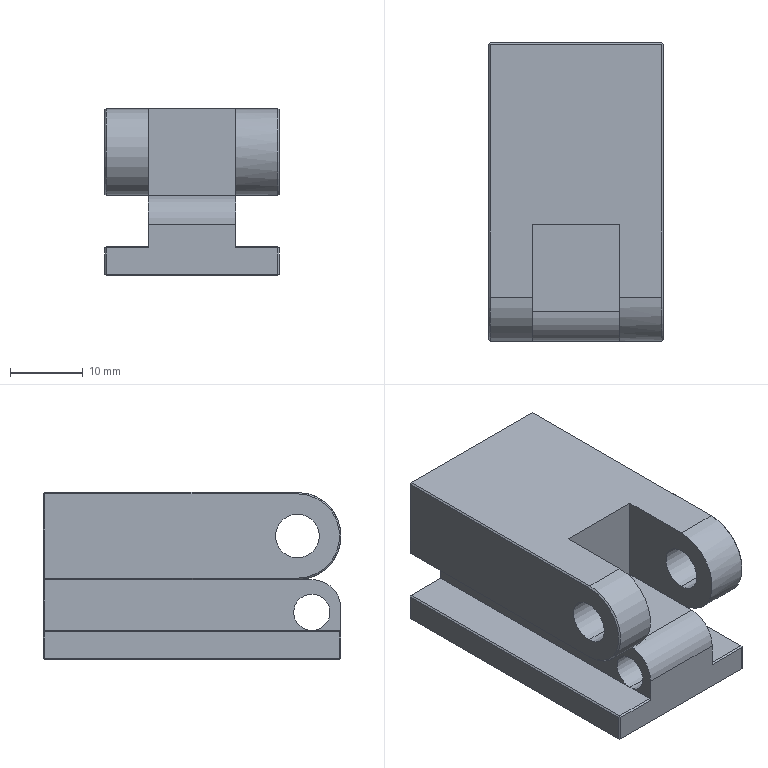Part | STEP file | 2009 | 1 solid | 55 faces | box 24 x 41 x 23 mm | volume 16072 mm3 | plane 43 | cylinder 9 | cone 3 | commonest cylinder face diameters 6 x4 5 x2 12 x2 8 x1